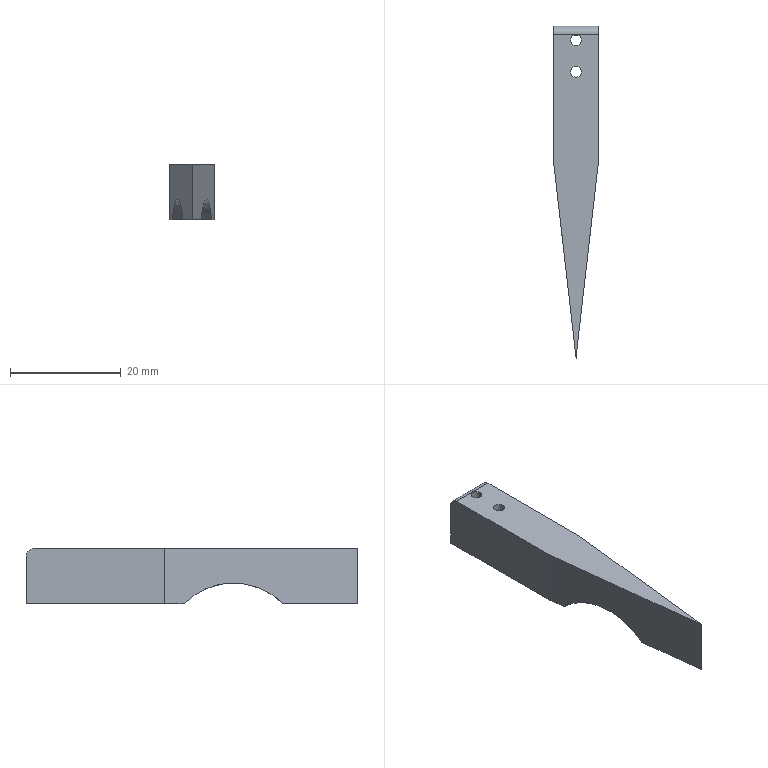Part | SolidWorks | features Cut 1, Extrusion 1, Fillet 1, ICE 1 | 1 solid | 14 faces | box 8 x 60 x 10 mm | volume 3101 mm3 | plane 8 | cylinder 6 | commonest cylinder face diameters 1.95 x4 3 x1 25 x1
STEP:
#1=CARTESIAN_POINT('',(-0.975,-8.284,0.));
#2=VERTEX_POINT('',#1);
#3=CARTESIAN_POINT('',(0.975,-8.284,0.));
#4=VERTEX_POINT('',#3);
#5=CARTESIAN_POINT('',(0.,-8.284,0.));
#6=DIRECTION('',(0.,0.,1.));
#7=DIRECTION('',(1.,0.,0.));
#8=AXIS2_PLACEMENT_3D('',#5,#6,#7);
#9=CIRCLE('',#8,0.975);
#10=EDGE_CURVE('',#2,#4,#9,.T.);
#11=ORIENTED_EDGE('',*,*,#10,.F.);
#12=CARTESIAN_POINT('',(-0.975,-8.284,10.));
#13=VERTEX_POINT('',#12);
#14=CARTESIAN_POINT('',(-0.975,-8.284,0.));
#15=DIRECTION('',(0.,0.,1.));
#16=VECTOR('',#15,1000.);
#17=LINE('',#14,#16);
#18=EDGE_CURVE('',#2,#13,#17,.T.);
#19=ORIENTED_EDGE('',*,*,#18,.T.);
#20=CARTESIAN_POINT('',(0.975,-8.284,10.));
#21=VERTEX_POINT('',#20);
#22=CARTESIAN_POINT('',(0.,-8.284,10.));
#23=DIRECTION('',(0.,0.,1.));
#24=DIRECTION('',(1.,0.,0.));
#25=AXIS2_PLACEMENT_3D('',#22,#23,#24);
#26=CIRCLE('',#25,0.975);
#27=EDGE_CURVE('',#13,#21,#26,.T.);
#28=ORIENTED_EDGE('',*,*,#27,.T.);
#29=CARTESIAN_POINT('',(0.975,-8.284,0.));
#30=DIRECTION('',(0.,0.,1.));
#31=VECTOR('',#30,1000.);
#32=LINE('',#29,#31);
#33=EDGE_CURVE('',#4,#21,#32,.T.);
#34=ORIENTED_EDGE('',*,*,#33,.F.);
#35=EDGE_LOOP('',(#11,#19,#28,#34));
#36=FACE_OUTER_BOUND('',#35,.T.);
#37=CARTESIAN_POINT('',(0.,-8.284,0.));
#38=DIRECTION('',(0.,0.,1.));
#39=DIRECTION('',(1.,0.,0.));
#40=AXIS2_PLACEMENT_3D('',#37,#38,#39);
#41=CYLINDRICAL_SURFACE('',#40,0.975);
#42=ADVANCED_FACE('',(#36),#41,.F.);
#43=CARTESIAN_POINT('',(-0.975,-2.584,0.));
#44=VERTEX_POINT('',#43);
#45=CARTESIAN_POINT('',(0.975,-2.584,0.));
#46=VERTEX_POINT('',#45);
#47=CARTESIAN_POINT('',(0.,-2.584,0.));
#48=DIRECTION('',(0.,0.,1.));
#49=DIRECTION('',(1.,0.,0.));
#50=AXIS2_PLACEMENT_3D('',#47,#48,#49);
#51=CIRCLE('',#50,0.975);
#52=EDGE_CURVE('',#44,#46,#51,.T.);
#53=ORIENTED_EDGE('',*,*,#52,.F.);
#54=CARTESIAN_POINT('',(-0.975,-2.584,10.));
#55=VERTEX_POINT('',#54);
#56=CARTESIAN_POINT('',(-0.975,-2.584,0.));
#57=DIRECTION('',(0.,0.,1.));
#58=VECTOR('',#57,1000.);
#59=LINE('',#56,#58);
#60=EDGE_CURVE('',#44,#55,#59,.T.);
#61=ORIENTED_EDGE('',*,*,#60,.T.);
#62=CARTESIAN_POINT('',(0.975,-2.584,10.));
#63=VERTEX_POINT('',#62);
#64=CARTESIAN_POINT('',(0.,-2.584,10.));
#65=DIRECTION('',(0.,0.,1.));
#66=DIRECTION('',(1.,0.,0.));
#67=AXIS2_PLACEMENT_3D('',#64,#65,#66);
#68=CIRCLE('',#67,0.975);
#69=EDGE_CURVE('',#55,#63,#68,.T.);
#70=ORIENTED_EDGE('',*,*,#69,.T.);
#71=CARTESIAN_POINT('',(0.975,-2.584,0.));
#72=DIRECTION('',(0.,0.,1.));
#73=VECTOR('',#72,1000.);
#74=LINE('',#71,#73);
#75=EDGE_CURVE('',#46,#63,#74,.T.);
#76=ORIENTED_EDGE('',*,*,#75,.F.);
#77=EDGE_LOOP('',(#53,#61,#70,#76));
#78=FACE_OUTER_BOUND('',#77,.T.);
#79=CARTESIAN_POINT('',(0.,-2.584,0.));
#80=DIRECTION('',(0.,0.,1.));
#81=DIRECTION('',(1.,0.,0.));
#82=AXIS2_PLACEMENT_3D('',#79,#80,#81);
#83=CYLINDRICAL_SURFACE('',#82,0.975);
#84=ADVANCED_FACE('',(#78),#83,.F.);
#85=CARTESIAN_POINT('',(0.,-2.584,0.));
#86=DIRECTION('',(0.,0.,1.));
#87=DIRECTION('',(1.,0.,0.));
#88=AXIS2_PLACEMENT_3D('',#85,#86,#87);
#89=CIRCLE('',#88,0.975);
#90=EDGE_CURVE('',#46,#44,#89,.T.);
#91=ORIENTED_EDGE('',*,*,#90,.T.);
#92=ORIENTED_EDGE('',*,*,#52,.T.);
#93=EDGE_LOOP('',(#91,#92));
#94=FACE_BOUND('',#93,.T.);
#95=CARTESIAN_POINT('',(0.,-8.284,0.));
#96=DIRECTION('',(0.,0.,1.));
#97=DIRECTION('',(1.,0.,0.));
#98=AXIS2_PLACEMENT_3D('',#95,#96,#97);
#99=CIRCLE('',#98,0.975);
#100=EDGE_CURVE('',#4,#2,#99,.T.);
#101=ORIENTED_EDGE('',*,*,#100,.T.);
#102=ORIENTED_EDGE('',*,*,#10,.T.);
#103=EDGE_LOOP('',(#101,#102));
#104=FACE_BOUND('',#103,.T.);
#105=CARTESIAN_POINT('',(3.589,-28.593,0.));
#106=VERTEX_POINT('',#105);
#107=CARTESIAN_POINT('',(4.,-25.,0.));
#108=VERTEX_POINT('',#107);
#109=CARTESIAN_POINT('',(4.,-25.,0.));
#110=DIRECTION('',(0.1135,0.9935,0.));
#111=VECTOR('',#110,1000.);
#112=LINE('',#109,#111);
#113=EDGE_CURVE('',#106,#108,#112,.T.);
#114=ORIENTED_EDGE('',*,*,#113,.F.);
#115=CARTESIAN_POINT('',(-3.589,-28.593,0.));
#116=VERTEX_POINT('',#115);
#117=CARTESIAN_POINT('',(4.,-28.593,0.));
#118=DIRECTION('',(-1.,0.,0.));
#119=VECTOR('',#118,1000.);
#120=LINE('',#117,#119);
#121=EDGE_CURVE('',#106,#116,#120,.T.);
#122=ORIENTED_EDGE('',*,*,#121,.T.);
#123=CARTESIAN_POINT('',(-4.,-25.,0.));
#124=VERTEX_POINT('',#123);
#125=CARTESIAN_POINT('',(-4.,-25.,0.));
#126=DIRECTION('',(0.1135,-0.9935,0.));
#127=VECTOR('',#126,1000.);
#128=LINE('',#125,#127);
#129=EDGE_CURVE('',#124,#116,#128,.T.);
#130=ORIENTED_EDGE('',*,*,#129,.F.);
#131=CARTESIAN_POINT('',(-4.,0.,0.));
#132=VERTEX_POINT('',#131);
#133=CARTESIAN_POINT('',(-4.,0.,0.));
#134=DIRECTION('',(0.,-1.,0.));
#135=VECTOR('',#134,1000.);
#136=LINE('',#133,#135);
#137=EDGE_CURVE('',#132,#124,#136,.T.);
#138=ORIENTED_EDGE('',*,*,#137,.F.);
#139=CARTESIAN_POINT('',(4.,0.,0.));
#140=VERTEX_POINT('',#139);
#141=CARTESIAN_POINT('',(-4.,0.,0.));
#142=DIRECTION('',(-1.,0.,0.));
#143=VECTOR('',#142,1000.);
#144=LINE('',#141,#143);
#145=EDGE_CURVE('',#140,#132,#144,.T.);
#146=ORIENTED_EDGE('',*,*,#145,.F.);
#147=CARTESIAN_POINT('',(4.,-25.,0.));
#148=DIRECTION('',(0.,1.,0.));
#149=VECTOR('',#148,1000.);
#150=LINE('',#147,#149);
#151=EDGE_CURVE('',#108,#140,#150,.T.);
#152=ORIENTED_EDGE('',*,*,#151,.F.);
#153=EDGE_LOOP('',(#114,#122,#130,#138,#146,#152));
#154=FACE_OUTER_BOUND('',#153,.T.);
#155=CARTESIAN_POINT('',(0.,0.,0.));
#156=DIRECTION('',(0.,0.,1.));
#157=DIRECTION('',(1.,0.,0.));
#158=AXIS2_PLACEMENT_3D('',#155,#156,#157);
#159=PLANE('',#158);
#160=ADVANCED_FACE('',(#94,#104,#154),#159,.F.);
#161=CARTESIAN_POINT('',(0.,-60.,0.));
#162=VERTEX_POINT('',#161);
#163=CARTESIAN_POINT('',(1.553,-46.407,0.));
#164=VERTEX_POINT('',#163);
#165=CARTESIAN_POINT('',(4.,-25.,0.));
#166=DIRECTION('',(0.1135,0.9935,0.));
#167=VECTOR('',#166,1000.);
#168=LINE('',#165,#167);
#169=EDGE_CURVE('',#162,#164,#168,.T.);
#170=ORIENTED_EDGE('',*,*,#169,.T.);
#171=CARTESIAN_POINT('',(1.553,-46.407,0.));
#172=CARTESIAN_POINT('',(2.148,-41.206,5.282));
#173=CARTESIAN_POINT('',(2.995,-33.794,5.282));
#174=CARTESIAN_POINT('',(3.589,-28.593,0.));
#175=(BOUNDED_CURVE()B_SPLINE_CURVE(3,(#171,#172,#173,#174),.UNSPECIFIED.,.F.,.F.)B_SPLINE_CURVE_WITH_KNOTS((4,4),(0.7776,2.364),.UNSPECIFIED.)CURVE()GEOMETRIC_REPRESENTATION_ITEM()RATIONAL_B_SPLINE_CURVE((1.,0.8011,0.8011,1.))REPRESENTATION_ITEM(''));
#176=EDGE_CURVE('',#164,#106,#175,.T.);
#177=ORIENTED_EDGE('',*,*,#176,.T.);
#178=ORIENTED_EDGE('',*,*,#113,.T.);
#179=CARTESIAN_POINT('',(4.,-25.,10.));
#180=VERTEX_POINT('',#179);
#181=CARTESIAN_POINT('',(4.,-25.,10.));
#182=DIRECTION('',(0.,0.,-1.));
#183=VECTOR('',#182,1000.);
#184=LINE('',#181,#183);
#185=EDGE_CURVE('',#180,#108,#184,.T.);
#186=ORIENTED_EDGE('',*,*,#185,.F.);
#187=CARTESIAN_POINT('',(0.,-60.,10.));
#188=VERTEX_POINT('',#187);
#189=CARTESIAN_POINT('',(4.,-25.,10.));
#190=DIRECTION('',(0.1135,0.9935,0.));
#191=VECTOR('',#190,1000.);
#192=LINE('',#189,#191);
#193=EDGE_CURVE('',#188,#180,#192,.T.);
#194=ORIENTED_EDGE('',*,*,#193,.F.);
#195=CARTESIAN_POINT('',(0.,-60.,10.));
#196=DIRECTION('',(0.,0.,-1.));
#197=VECTOR('',#196,1000.);
#198=LINE('',#195,#197);
#199=EDGE_CURVE('',#188,#162,#198,.T.);
#200=ORIENTED_EDGE('',*,*,#199,.T.);
#201=EDGE_LOOP('',(#170,#177,#178,#186,#194,#200));
#202=FACE_OUTER_BOUND('',#201,.T.);
#203=CARTESIAN_POINT('',(4.,-25.,10.));
#204=DIRECTION('',(-0.9935,0.1135,0.));
#205=DIRECTION('',(-0.1135,-0.9935,0.));
#206=AXIS2_PLACEMENT_3D('',#203,#204,#205);
#207=PLANE('',#206);
#208=ADVANCED_FACE('',(#202),#207,.F.);
#209=CARTESIAN_POINT('',(4.,0.,8.5));
#210=VERTEX_POINT('',#209);
#211=CARTESIAN_POINT('',(4.,0.,10.));
#212=DIRECTION('',(0.,0.,-1.));
#213=VECTOR('',#212,1000.);
#214=LINE('',#211,#213);
#215=EDGE_CURVE('',#210,#140,#214,.T.);
#216=ORIENTED_EDGE('',*,*,#215,.F.);
#217=CARTESIAN_POINT('',(4.,-1.5,10.));
#218=VERTEX_POINT('',#217);
#219=CARTESIAN_POINT('',(4.,-1.5,8.5));
#220=DIRECTION('',(1.,0.,0.));
#221=DIRECTION('',(0.,-1.,0.));
#222=AXIS2_PLACEMENT_3D('',#219,#220,#221);
#223=CIRCLE('',#222,1.5);
#224=EDGE_CURVE('',#210,#218,#223,.T.);
#225=ORIENTED_EDGE('',*,*,#224,.T.);
#226=CARTESIAN_POINT('',(4.,-25.,10.));
#227=DIRECTION('',(0.,1.,0.));
#228=VECTOR('',#227,1000.);
#229=LINE('',#226,#228);
#230=EDGE_CURVE('',#180,#218,#229,.T.);
#231=ORIENTED_EDGE('',*,*,#230,.F.);
#232=ORIENTED_EDGE('',*,*,#185,.T.);
#233=ORIENTED_EDGE('',*,*,#151,.T.);
#234=EDGE_LOOP('',(#216,#225,#231,#232,#233));
#235=FACE_OUTER_BOUND('',#234,.T.);
#236=CARTESIAN_POINT('',(4.,-25.,10.));
#237=DIRECTION('',(-1.,0.,0.));
#238=DIRECTION('',(0.,-1.,0.));
#239=AXIS2_PLACEMENT_3D('',#236,#237,#238);
#240=PLANE('',#239);
#241=ADVANCED_FACE('',(#235),#240,.F.);
#242=CARTESIAN_POINT('',(-4.,0.,8.5));
#243=VERTEX_POINT('',#242);
#244=CARTESIAN_POINT('',(-4.,0.,10.));
#245=DIRECTION('',(0.,0.,-1.));
#246=VECTOR('',#245,1000.);
#247=LINE('',#244,#246);
#248=EDGE_CURVE('',#243,#132,#247,.T.);
#249=ORIENTED_EDGE('',*,*,#248,.F.);
#250=CARTESIAN_POINT('',(4.,0.,8.5));
#251=DIRECTION('',(1.,0.,0.));
#252=VECTOR('',#251,1000.);
#253=LINE('',#250,#252);
#254=EDGE_CURVE('',#243,#210,#253,.T.);
#255=ORIENTED_EDGE('',*,*,#254,.T.);
#256=ORIENTED_EDGE('',*,*,#215,.T.);
#257=ORIENTED_EDGE('',*,*,#145,.T.);
#258=EDGE_LOOP('',(#249,#255,#256,#257));
#259=FACE_OUTER_BOUND('',#258,.T.);
#260=CARTESIAN_POINT('',(-4.,0.,10.));
#261=DIRECTION('',(0.,-1.,0.));
#262=DIRECTION('',(1.,0.,0.));
#263=AXIS2_PLACEMENT_3D('',#260,#261,#262);
#264=PLANE('',#263);
#265=ADVANCED_FACE('',(#259),#264,.F.);
#266=CARTESIAN_POINT('',(-4.,-1.5,10.));
#267=VERTEX_POINT('',#266);
#268=CARTESIAN_POINT('',(-4.,-25.,10.));
#269=VERTEX_POINT('',#268);
#270=CARTESIAN_POINT('',(-4.,0.,10.));
#271=DIRECTION('',(0.,-1.,0.));
#272=VECTOR('',#271,1000.);
#273=LINE('',#270,#272);
#274=EDGE_CURVE('',#267,#269,#273,.T.);
#275=ORIENTED_EDGE('',*,*,#274,.F.);
#276=CARTESIAN_POINT('',(-4.,-1.5,8.5));
#277=DIRECTION('',(-1.,0.,0.));
#278=DIRECTION('',(0.,1.,0.));
#279=AXIS2_PLACEMENT_3D('',#276,#277,#278);
#280=CIRCLE('',#279,1.5);
#281=EDGE_CURVE('',#267,#243,#280,.T.);
#282=ORIENTED_EDGE('',*,*,#281,.T.);
#283=ORIENTED_EDGE('',*,*,#248,.T.);
#284=ORIENTED_EDGE('',*,*,#137,.T.);
#285=CARTESIAN_POINT('',(-4.,-25.,10.));
#286=DIRECTION('',(0.,0.,-1.));
#287=VECTOR('',#286,1000.);
#288=LINE('',#285,#287);
#289=EDGE_CURVE('',#269,#124,#288,.T.);
#290=ORIENTED_EDGE('',*,*,#289,.F.);
#291=EDGE_LOOP('',(#275,#282,#283,#284,#290));
#292=FACE_OUTER_BOUND('',#291,.T.);
#293=CARTESIAN_POINT('',(-4.,0.,10.));
#294=DIRECTION('',(1.,0.,0.));
#295=DIRECTION('',(0.,1.,0.));
#296=AXIS2_PLACEMENT_3D('',#293,#294,#295);
#297=PLANE('',#296);
#298=ADVANCED_FACE('',(#292),#297,.F.);
#299=ORIENTED_EDGE('',*,*,#129,.T.);
#300=CARTESIAN_POINT('',(-1.553,-46.407,0.));
#301=VERTEX_POINT('',#300);
#302=CARTESIAN_POINT('',(-3.589,-28.593,0.));
#303=CARTESIAN_POINT('',(-2.995,-33.794,5.282));
#304=CARTESIAN_POINT('',(-2.148,-41.206,5.282));
#305=CARTESIAN_POINT('',(-1.553,-46.407,0.));
#306=(BOUNDED_CURVE()B_SPLINE_CURVE(3,(#302,#303,#304,#305),.UNSPECIFIED.,.F.,.F.)B_SPLINE_CURVE_WITH_KNOTS((4,4),(0.7776,2.364),.UNSPECIFIED.)CURVE()GEOMETRIC_REPRESENTATION_ITEM()RATIONAL_B_SPLINE_CURVE((1.,0.8011,0.8011,1.))REPRESENTATION_ITEM(''));
#307=EDGE_CURVE('',#116,#301,#306,.T.);
#308=ORIENTED_EDGE('',*,*,#307,.T.);
#309=CARTESIAN_POINT('',(-4.,-25.,0.));
#310=DIRECTION('',(0.1135,-0.9935,0.));
#311=VECTOR('',#310,1000.);
#312=LINE('',#309,#311);
#313=EDGE_CURVE('',#301,#162,#312,.T.);
#314=ORIENTED_EDGE('',*,*,#313,.T.);
#315=ORIENTED_EDGE('',*,*,#199,.F.);
#316=CARTESIAN_POINT('',(-4.,-25.,10.));
#317=DIRECTION('',(0.1135,-0.9935,0.));
#318=VECTOR('',#317,1000.);
#319=LINE('',#316,#318);
#320=EDGE_CURVE('',#269,#188,#319,.T.);
#321=ORIENTED_EDGE('',*,*,#320,.F.);
#322=ORIENTED_EDGE('',*,*,#289,.T.);
#323=EDGE_LOOP('',(#299,#308,#314,#315,#321,#322));
#324=FACE_OUTER_BOUND('',#323,.T.);
#325=CARTESIAN_POINT('',(-4.,-25.,10.));
#326=DIRECTION('',(0.9935,0.1135,0.));
#327=DIRECTION('',(-0.1135,0.9935,0.));
#328=AXIS2_PLACEMENT_3D('',#325,#326,#327);
#329=PLANE('',#328);
#330=ADVANCED_FACE('',(#324),#329,.F.);
#331=CARTESIAN_POINT('',(0.,-8.284,10.));
#332=DIRECTION('',(0.,0.,1.));
#333=DIRECTION('',(1.,0.,0.));
#334=AXIS2_PLACEMENT_3D('',#331,#332,#333);
#335=CIRCLE('',#334,0.975);
#336=EDGE_CURVE('',#21,#13,#335,.T.);
#337=ORIENTED_EDGE('',*,*,#336,.F.);
#338=ORIENTED_EDGE('',*,*,#27,.F.);
#339=EDGE_LOOP('',(#337,#338));
#340=FACE_BOUND('',#339,.T.);
#341=CARTESIAN_POINT('',(0.,-2.584,10.));
#342=DIRECTION('',(0.,0.,1.));
#343=DIRECTION('',(1.,0.,0.));
#344=AXIS2_PLACEMENT_3D('',#341,#342,#343);
#345=CIRCLE('',#344,0.975);
#346=EDGE_CURVE('',#63,#55,#345,.T.);
#347=ORIENTED_EDGE('',*,*,#346,.F.);
#348=ORIENTED_EDGE('',*,*,#69,.F.);
#349=EDGE_LOOP('',(#347,#348));
#350=FACE_BOUND('',#349,.T.);
#351=ORIENTED_EDGE('',*,*,#230,.T.);
#352=CARTESIAN_POINT('',(-4.,-1.5,10.));
#353=DIRECTION('',(-1.,0.,0.));
#354=VECTOR('',#353,1000.);
#355=LINE('',#352,#354);
#356=EDGE_CURVE('',#218,#267,#355,.T.);
#357=ORIENTED_EDGE('',*,*,#356,.T.);
#358=ORIENTED_EDGE('',*,*,#274,.T.);
#359=ORIENTED_EDGE('',*,*,#320,.T.);
#360=ORIENTED_EDGE('',*,*,#193,.T.);
#361=EDGE_LOOP('',(#351,#357,#358,#359,#360));
#362=FACE_OUTER_BOUND('',#361,.T.);
#363=CARTESIAN_POINT('',(0.,0.,10.));
#364=DIRECTION('',(0.,0.,1.));
#365=DIRECTION('',(1.,0.,0.));
#366=AXIS2_PLACEMENT_3D('',#363,#364,#365);
#367=PLANE('',#366);
#368=ADVANCED_FACE('',(#340,#350,#362),#367,.T.);
#369=ORIENTED_EDGE('',*,*,#313,.F.);
#370=CARTESIAN_POINT('',(4.,-46.407,0.));
#371=DIRECTION('',(1.,0.,0.));
#372=VECTOR('',#371,1000.);
#373=LINE('',#370,#372);
#374=EDGE_CURVE('',#301,#164,#373,.T.);
#375=ORIENTED_EDGE('',*,*,#374,.T.);
#376=ORIENTED_EDGE('',*,*,#169,.F.);
#377=EDGE_LOOP('',(#369,#375,#376));
#378=FACE_OUTER_BOUND('',#377,.T.);
#379=CARTESIAN_POINT('',(0.,0.,0.));
#380=DIRECTION('',(0.,0.,1.));
#381=DIRECTION('',(1.,0.,0.));
#382=AXIS2_PLACEMENT_3D('',#379,#380,#381);
#383=PLANE('',#382);
#384=ADVANCED_FACE('',(#378),#383,.F.);
#385=ORIENTED_EDGE('',*,*,#60,.F.);
#386=ORIENTED_EDGE('',*,*,#90,.F.);
#387=ORIENTED_EDGE('',*,*,#75,.T.);
#388=ORIENTED_EDGE('',*,*,#346,.T.);
#389=EDGE_LOOP('',(#385,#386,#387,#388));
#390=FACE_OUTER_BOUND('',#389,.T.);
#391=CARTESIAN_POINT('',(0.,-2.584,0.));
#392=DIRECTION('',(0.,0.,1.));
#393=DIRECTION('',(1.,0.,0.));
#394=AXIS2_PLACEMENT_3D('',#391,#392,#393);
#395=CYLINDRICAL_SURFACE('',#394,0.975);
#396=ADVANCED_FACE('',(#390),#395,.F.);
#397=ORIENTED_EDGE('',*,*,#18,.F.);
#398=ORIENTED_EDGE('',*,*,#100,.F.);
#399=ORIENTED_EDGE('',*,*,#33,.T.);
#400=ORIENTED_EDGE('',*,*,#336,.T.);
#401=EDGE_LOOP('',(#397,#398,#399,#400));
#402=FACE_OUTER_BOUND('',#401,.T.);
#403=CARTESIAN_POINT('',(0.,-8.284,0.));
#404=DIRECTION('',(0.,0.,1.));
#405=DIRECTION('',(1.,0.,0.));
#406=AXIS2_PLACEMENT_3D('',#403,#404,#405);
#407=CYLINDRICAL_SURFACE('',#406,0.975);
#408=ADVANCED_FACE('',(#402),#407,.F.);
#409=ORIENTED_EDGE('',*,*,#224,.F.);
#410=ORIENTED_EDGE('',*,*,#254,.F.);
#411=ORIENTED_EDGE('',*,*,#281,.F.);
#412=ORIENTED_EDGE('',*,*,#356,.F.);
#413=EDGE_LOOP('',(#409,#410,#411,#412));
#414=FACE_OUTER_BOUND('',#413,.T.);
#415=CARTESIAN_POINT('',(0.,-1.5,8.5));
#416=DIRECTION('',(1.,0.,0.));
#417=DIRECTION('',(0.,1.,0.));
#418=AXIS2_PLACEMENT_3D('',#415,#416,#417);
#419=CYLINDRICAL_SURFACE('',#418,1.5);
#420=ADVANCED_FACE('',(#414),#419,.T.);
#421=ORIENTED_EDGE('',*,*,#176,.F.);
#422=ORIENTED_EDGE('',*,*,#374,.F.);
#423=ORIENTED_EDGE('',*,*,#307,.F.);
#424=ORIENTED_EDGE('',*,*,#121,.F.);
#425=EDGE_LOOP('',(#421,#422,#423,#424));
#426=FACE_OUTER_BOUND('',#425,.T.);
#427=CARTESIAN_POINT('',(4.,-37.5,-8.77));
#428=DIRECTION('',(-1.,0.,0.));
#429=DIRECTION('',(0.,-1.,0.));
#430=AXIS2_PLACEMENT_3D('',#427,#428,#429);
#431=CYLINDRICAL_SURFACE('',#430,12.5);
#432=ADVANCED_FACE('',(#426),#431,.F.);
#433=CLOSED_SHELL('',(#42,#84,#160,#208,#241,#265,#298,#330,#368,#384,#396,#408,#420,#432));
#434=MANIFOLD_SOLID_BREP('',#433);
#435=CARTESIAN_POINT('',(0.,0.,0.));
#436=DIRECTION('',(0.,0.,1.));
#437=DIRECTION('',(1.,0.,0.));
#438=AXIS2_PLACEMENT_3D('',#435,#436,#437);
#439=(LENGTH_UNIT()NAMED_UNIT(*)SI_UNIT(.MILLI.,.METRE.));
#440=UNCERTAINTY_MEASURE_WITH_UNIT(LENGTH_MEASURE(0.00001),#439,'','');
#441=(NAMED_UNIT(*)PLANE_ANGLE_UNIT()SI_UNIT($,.RADIAN.));
#442=(NAMED_UNIT(*)SI_UNIT($,.STERADIAN.)SOLID_ANGLE_UNIT());
#443=(GEOMETRIC_REPRESENTATION_CONTEXT(3)GLOBAL_UNCERTAINTY_ASSIGNED_CONTEXT((#440))GLOBAL_UNIT_ASSIGNED_CONTEXT((#439,#441,#442))REPRESENTATION_CONTEXT('',''));
#444=ADVANCED_BREP_SHAPE_REPRESENTATION('',(#434,#438),#443);